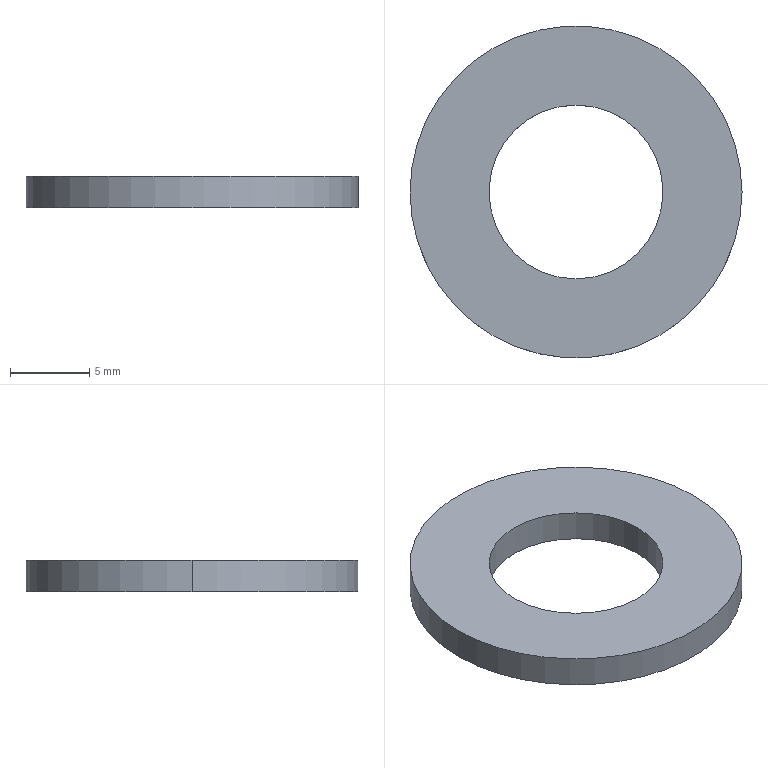Part | STEP file | Surge arrester washer | 1 solid | 6 faces | box 21 x 21 x 2 mm | volume 502.655 mm3 | cylinder 4 | plane 2 | commonest cylinder face diameters 11 x2 21 x2
STEP:
#1=CARTESIAN_POINT('',(0.,0.,0.));
#2=DIRECTION('',(0.,0.,1.));
#3=DIRECTION('',(1.,0.,0.));
#4=AXIS2_PLACEMENT_3D('',#1,#2,#3);
#5=CARTESIAN_POINT('',(-5.5,0.,2.));
#6=VERTEX_POINT('',#5);
#7=CARTESIAN_POINT('',(-5.5,0.,0.));
#8=VERTEX_POINT('',#7);
#9=CARTESIAN_POINT('',(-5.5,0.,2.));
#10=DIRECTION('',(0.,0.,-1.));
#11=VECTOR('',#10,1.);
#12=LINE('',#9,#11);
#13=CARTESIAN_POINT('',(0.,0.,2.));
#14=DIRECTION('',(0.,0.,-1.));
#15=DIRECTION('',(-1.,0.,0.));
#16=AXIS2_PLACEMENT_3D('',#13,#14,#15);
#17=CYLINDRICAL_SURFACE('',#16,5.5);
#18=CARTESIAN_POINT('',(6.283,0.));
#19=DIRECTION('',(0.,1.));
#20=VECTOR('',#19,1.);
#21=LINE('',#18,#20);
#22=(GEOMETRIC_REPRESENTATION_CONTEXT(2)PARAMETRIC_REPRESENTATION_CONTEXT()REPRESENTATION_CONTEXT('',''));
#23=DEFINITIONAL_REPRESENTATION('',(#21),#22);
#24=PCURVE('',#17,#23);
#25=CARTESIAN_POINT('',(0.,0.,2.));
#26=DIRECTION('',(0.,0.,-1.));
#27=DIRECTION('',(-1.,0.,0.));
#28=AXIS2_PLACEMENT_3D('',#25,#26,#27);
#29=CYLINDRICAL_SURFACE('',#28,5.5);
#30=CARTESIAN_POINT('',(0.,0.));
#31=DIRECTION('',(0.,1.));
#32=VECTOR('',#31,1.);
#33=LINE('',#30,#32);
#34=(GEOMETRIC_REPRESENTATION_CONTEXT(2)PARAMETRIC_REPRESENTATION_CONTEXT()REPRESENTATION_CONTEXT('',''));
#35=DEFINITIONAL_REPRESENTATION('',(#33),#34);
#36=PCURVE('',#29,#35);
#37=SURFACE_CURVE('',#12,(#24,#36),.PCURVE_S1.);
#38=EDGE_CURVE('',#6,#8,#37,.T.);
#39=ORIENTED_EDGE('',*,*,#38,.T.);
#40=CARTESIAN_POINT('',(5.5,0.,0.));
#41=VERTEX_POINT('',#40);
#42=CARTESIAN_POINT('',(0.,0.,0.));
#43=DIRECTION('',(0.,0.,1.));
#44=DIRECTION('',(1.,0.,0.));
#45=AXIS2_PLACEMENT_3D('',#42,#43,#44);
#46=CIRCLE('',#45,5.5);
#47=CARTESIAN_POINT('',(9.425,2.));
#48=DIRECTION('',(-1.,0.));
#49=VECTOR('',#48,1.);
#50=LINE('',#47,#49);
#51=(GEOMETRIC_REPRESENTATION_CONTEXT(2)PARAMETRIC_REPRESENTATION_CONTEXT()REPRESENTATION_CONTEXT('',''));
#52=DEFINITIONAL_REPRESENTATION('',(#50),#51);
#53=PCURVE('',#17,#52);
#54=CARTESIAN_POINT('',(0.,0.,0.));
#55=DIRECTION('',(0.,0.,1.));
#56=DIRECTION('',(1.,0.,0.));
#57=AXIS2_PLACEMENT_3D('',#54,#55,#56);
#58=PLANE('',#57);
#59=CARTESIAN_POINT('',(0.,0.));
#60=DIRECTION('',(1.,0.));
#61=AXIS2_PLACEMENT_2D('',#59,#60);
#62=CIRCLE('',#61,5.5);
#63=(GEOMETRIC_REPRESENTATION_CONTEXT(2)PARAMETRIC_REPRESENTATION_CONTEXT()REPRESENTATION_CONTEXT('',''));
#64=DEFINITIONAL_REPRESENTATION('',(#62),#63);
#65=PCURVE('',#58,#64);
#66=SURFACE_CURVE('',#46,(#53,#65),.PCURVE_S1.);
#67=EDGE_CURVE('',#8,#41,#66,.T.);
#68=ORIENTED_EDGE('',*,*,#67,.T.);
#69=CARTESIAN_POINT('',(5.5,0.,2.));
#70=VERTEX_POINT('',#69);
#71=CARTESIAN_POINT('',(5.5,0.,2.));
#72=DIRECTION('',(0.,0.,-1.));
#73=VECTOR('',#72,1.);
#74=LINE('',#71,#73);
#75=CARTESIAN_POINT('',(3.142,0.));
#76=DIRECTION('',(0.,1.));
#77=VECTOR('',#76,1.);
#78=LINE('',#75,#77);
#79=(GEOMETRIC_REPRESENTATION_CONTEXT(2)PARAMETRIC_REPRESENTATION_CONTEXT()REPRESENTATION_CONTEXT('',''));
#80=DEFINITIONAL_REPRESENTATION('',(#78),#79);
#81=PCURVE('',#17,#80);
#82=CARTESIAN_POINT('',(3.142,0.));
#83=DIRECTION('',(0.,1.));
#84=VECTOR('',#83,1.);
#85=LINE('',#82,#84);
#86=(GEOMETRIC_REPRESENTATION_CONTEXT(2)PARAMETRIC_REPRESENTATION_CONTEXT()REPRESENTATION_CONTEXT('',''));
#87=DEFINITIONAL_REPRESENTATION('',(#85),#86);
#88=PCURVE('',#29,#87);
#89=SURFACE_CURVE('',#74,(#81,#88),.PCURVE_S1.);
#90=EDGE_CURVE('',#70,#41,#89,.T.);
#91=ORIENTED_EDGE('',*,*,#90,.F.);
#92=CARTESIAN_POINT('',(0.,0.,2.));
#93=DIRECTION('',(0.,0.,1.));
#94=DIRECTION('',(1.,0.,0.));
#95=AXIS2_PLACEMENT_3D('',#92,#93,#94);
#96=CIRCLE('',#95,5.5);
#97=CARTESIAN_POINT('',(9.425,0.));
#98=DIRECTION('',(-1.,0.));
#99=VECTOR('',#98,1.);
#100=LINE('',#97,#99);
#101=(GEOMETRIC_REPRESENTATION_CONTEXT(2)PARAMETRIC_REPRESENTATION_CONTEXT()REPRESENTATION_CONTEXT('',''));
#102=DEFINITIONAL_REPRESENTATION('',(#100),#101);
#103=PCURVE('',#17,#102);
#104=CARTESIAN_POINT('',(0.,0.,2.));
#105=DIRECTION('',(0.,0.,1.));
#106=DIRECTION('',(1.,0.,0.));
#107=AXIS2_PLACEMENT_3D('',#104,#105,#106);
#108=PLANE('',#107);
#109=CARTESIAN_POINT('',(0.,0.));
#110=DIRECTION('',(1.,0.));
#111=AXIS2_PLACEMENT_2D('',#109,#110);
#112=CIRCLE('',#111,5.5);
#113=(GEOMETRIC_REPRESENTATION_CONTEXT(2)PARAMETRIC_REPRESENTATION_CONTEXT()REPRESENTATION_CONTEXT('',''));
#114=DEFINITIONAL_REPRESENTATION('',(#112),#113);
#115=PCURVE('',#108,#114);
#116=SURFACE_CURVE('',#96,(#103,#115),.PCURVE_S1.);
#117=EDGE_CURVE('',#6,#70,#116,.T.);
#118=ORIENTED_EDGE('',*,*,#117,.F.);
#119=EDGE_LOOP('',(#39,#68,#91,#118));
#120=FACE_BOUND('',#119,.F.);
#121=ADVANCED_FACE('',(#120),#17,.F.);
#122=CARTESIAN_POINT('',(10.5,0.,2.));
#123=VERTEX_POINT('',#122);
#124=CARTESIAN_POINT('',(-10.5,0.,2.));
#125=VERTEX_POINT('',#124);
#126=CARTESIAN_POINT('',(0.,0.,2.));
#127=DIRECTION('',(0.,0.,1.));
#128=DIRECTION('',(1.,0.,0.));
#129=AXIS2_PLACEMENT_3D('',#126,#127,#128);
#130=CIRCLE('',#129,10.5);
#131=CARTESIAN_POINT('',(0.,0.,2.));
#132=DIRECTION('',(0.,0.,-1.));
#133=DIRECTION('',(-1.,0.,0.));
#134=AXIS2_PLACEMENT_3D('',#131,#132,#133);
#135=CYLINDRICAL_SURFACE('',#134,10.5);
#136=CARTESIAN_POINT('',(3.142,0.));
#137=DIRECTION('',(-1.,0.));
#138=VECTOR('',#137,1.);
#139=LINE('',#136,#138);
#140=(GEOMETRIC_REPRESENTATION_CONTEXT(2)PARAMETRIC_REPRESENTATION_CONTEXT()REPRESENTATION_CONTEXT('',''));
#141=DEFINITIONAL_REPRESENTATION('',(#139),#140);
#142=PCURVE('',#135,#141);
#143=CARTESIAN_POINT('',(0.,0.));
#144=DIRECTION('',(1.,0.));
#145=AXIS2_PLACEMENT_2D('',#143,#144);
#146=CIRCLE('',#145,10.5);
#147=(GEOMETRIC_REPRESENTATION_CONTEXT(2)PARAMETRIC_REPRESENTATION_CONTEXT()REPRESENTATION_CONTEXT('',''));
#148=DEFINITIONAL_REPRESENTATION('',(#146),#147);
#149=PCURVE('',#108,#148);
#150=SURFACE_CURVE('',#130,(#142,#149),.PCURVE_S1.);
#151=EDGE_CURVE('',#123,#125,#150,.T.);
#152=ORIENTED_EDGE('',*,*,#151,.F.);
#153=CARTESIAN_POINT('',(10.5,0.,0.));
#154=VERTEX_POINT('',#153);
#155=CARTESIAN_POINT('',(10.5,0.,2.));
#156=DIRECTION('',(0.,0.,-1.));
#157=VECTOR('',#156,1.);
#158=LINE('',#155,#157);
#159=CARTESIAN_POINT('',(3.142,0.));
#160=DIRECTION('',(0.,1.));
#161=VECTOR('',#160,1.);
#162=LINE('',#159,#161);
#163=(GEOMETRIC_REPRESENTATION_CONTEXT(2)PARAMETRIC_REPRESENTATION_CONTEXT()REPRESENTATION_CONTEXT('',''));
#164=DEFINITIONAL_REPRESENTATION('',(#162),#163);
#165=PCURVE('',#135,#164);
#166=CARTESIAN_POINT('',(0.,0.,2.));
#167=DIRECTION('',(0.,0.,-1.));
#168=DIRECTION('',(-1.,0.,0.));
#169=AXIS2_PLACEMENT_3D('',#166,#167,#168);
#170=CYLINDRICAL_SURFACE('',#169,10.5);
#171=CARTESIAN_POINT('',(3.142,0.));
#172=DIRECTION('',(0.,1.));
#173=VECTOR('',#172,1.);
#174=LINE('',#171,#173);
#175=(GEOMETRIC_REPRESENTATION_CONTEXT(2)PARAMETRIC_REPRESENTATION_CONTEXT()REPRESENTATION_CONTEXT('',''));
#176=DEFINITIONAL_REPRESENTATION('',(#174),#175);
#177=PCURVE('',#170,#176);
#178=SURFACE_CURVE('',#158,(#165,#177),.PCURVE_S1.);
#179=EDGE_CURVE('',#123,#154,#178,.T.);
#180=ORIENTED_EDGE('',*,*,#179,.T.);
#181=CARTESIAN_POINT('',(-10.5,0.,0.));
#182=VERTEX_POINT('',#181);
#183=CARTESIAN_POINT('',(0.,0.,0.));
#184=DIRECTION('',(0.,0.,1.));
#185=DIRECTION('',(1.,0.,0.));
#186=AXIS2_PLACEMENT_3D('',#183,#184,#185);
#187=CIRCLE('',#186,10.5);
#188=CARTESIAN_POINT('',(3.142,2.));
#189=DIRECTION('',(-1.,0.));
#190=VECTOR('',#189,1.);
#191=LINE('',#188,#190);
#192=(GEOMETRIC_REPRESENTATION_CONTEXT(2)PARAMETRIC_REPRESENTATION_CONTEXT()REPRESENTATION_CONTEXT('',''));
#193=DEFINITIONAL_REPRESENTATION('',(#191),#192);
#194=PCURVE('',#135,#193);
#195=CARTESIAN_POINT('',(0.,0.));
#196=DIRECTION('',(1.,0.));
#197=AXIS2_PLACEMENT_2D('',#195,#196);
#198=CIRCLE('',#197,10.5);
#199=(GEOMETRIC_REPRESENTATION_CONTEXT(2)PARAMETRIC_REPRESENTATION_CONTEXT()REPRESENTATION_CONTEXT('',''));
#200=DEFINITIONAL_REPRESENTATION('',(#198),#199);
#201=PCURVE('',#58,#200);
#202=SURFACE_CURVE('',#187,(#194,#201),.PCURVE_S1.);
#203=EDGE_CURVE('',#154,#182,#202,.T.);
#204=ORIENTED_EDGE('',*,*,#203,.T.);
#205=CARTESIAN_POINT('',(-10.5,0.,2.));
#206=DIRECTION('',(0.,0.,-1.));
#207=VECTOR('',#206,1.);
#208=LINE('',#205,#207);
#209=CARTESIAN_POINT('',(0.,0.));
#210=DIRECTION('',(0.,1.));
#211=VECTOR('',#210,1.);
#212=LINE('',#209,#211);
#213=(GEOMETRIC_REPRESENTATION_CONTEXT(2)PARAMETRIC_REPRESENTATION_CONTEXT()REPRESENTATION_CONTEXT('',''));
#214=DEFINITIONAL_REPRESENTATION('',(#212),#213);
#215=PCURVE('',#135,#214);
#216=CARTESIAN_POINT('',(6.283,0.));
#217=DIRECTION('',(0.,1.));
#218=VECTOR('',#217,1.);
#219=LINE('',#216,#218);
#220=(GEOMETRIC_REPRESENTATION_CONTEXT(2)PARAMETRIC_REPRESENTATION_CONTEXT()REPRESENTATION_CONTEXT('',''));
#221=DEFINITIONAL_REPRESENTATION('',(#219),#220);
#222=PCURVE('',#170,#221);
#223=SURFACE_CURVE('',#208,(#215,#222),.PCURVE_S1.);
#224=EDGE_CURVE('',#125,#182,#223,.T.);
#225=ORIENTED_EDGE('',*,*,#224,.F.);
#226=EDGE_LOOP('',(#152,#180,#204,#225));
#227=FACE_BOUND('',#226,.T.);
#228=ADVANCED_FACE('',(#227),#135,.T.);
#229=CARTESIAN_POINT('',(0.,0.,2.));
#230=DIRECTION('',(0.,0.,1.));
#231=DIRECTION('',(1.,0.,0.));
#232=AXIS2_PLACEMENT_3D('',#229,#230,#231);
#233=CIRCLE('',#232,10.5);
#234=CARTESIAN_POINT('',(0.,0.));
#235=DIRECTION('',(1.,0.));
#236=AXIS2_PLACEMENT_2D('',#234,#235);
#237=CIRCLE('',#236,10.5);
#238=(GEOMETRIC_REPRESENTATION_CONTEXT(2)PARAMETRIC_REPRESENTATION_CONTEXT()REPRESENTATION_CONTEXT('',''));
#239=DEFINITIONAL_REPRESENTATION('',(#237),#238);
#240=PCURVE('',#108,#239);
#241=CARTESIAN_POINT('',(9.425,0.));
#242=DIRECTION('',(-1.,0.));
#243=VECTOR('',#242,1.);
#244=LINE('',#241,#243);
#245=(GEOMETRIC_REPRESENTATION_CONTEXT(2)PARAMETRIC_REPRESENTATION_CONTEXT()REPRESENTATION_CONTEXT('',''));
#246=DEFINITIONAL_REPRESENTATION('',(#244),#245);
#247=PCURVE('',#170,#246);
#248=SURFACE_CURVE('',#233,(#240,#247),.PCURVE_S1.);
#249=EDGE_CURVE('',#125,#123,#248,.T.);
#250=ORIENTED_EDGE('',*,*,#249,.T.);
#251=ORIENTED_EDGE('',*,*,#151,.T.);
#252=EDGE_LOOP('',(#250,#251));
#253=FACE_BOUND('',#252,.T.);
#254=ORIENTED_EDGE('',*,*,#117,.F.);
#255=CARTESIAN_POINT('',(0.,0.,2.));
#256=DIRECTION('',(0.,0.,1.));
#257=DIRECTION('',(1.,0.,0.));
#258=AXIS2_PLACEMENT_3D('',#255,#256,#257);
#259=CIRCLE('',#258,5.5);
#260=CARTESIAN_POINT('',(0.,0.));
#261=DIRECTION('',(1.,0.));
#262=AXIS2_PLACEMENT_2D('',#260,#261);
#263=CIRCLE('',#262,5.5);
#264=(GEOMETRIC_REPRESENTATION_CONTEXT(2)PARAMETRIC_REPRESENTATION_CONTEXT()REPRESENTATION_CONTEXT('',''));
#265=DEFINITIONAL_REPRESENTATION('',(#263),#264);
#266=PCURVE('',#108,#265);
#267=CARTESIAN_POINT('',(3.142,0.));
#268=DIRECTION('',(-1.,0.));
#269=VECTOR('',#268,1.);
#270=LINE('',#267,#269);
#271=(GEOMETRIC_REPRESENTATION_CONTEXT(2)PARAMETRIC_REPRESENTATION_CONTEXT()REPRESENTATION_CONTEXT('',''));
#272=DEFINITIONAL_REPRESENTATION('',(#270),#271);
#273=PCURVE('',#29,#272);
#274=SURFACE_CURVE('',#259,(#266,#273),.PCURVE_S1.);
#275=EDGE_CURVE('',#70,#6,#274,.T.);
#276=ORIENTED_EDGE('',*,*,#275,.F.);
#277=EDGE_LOOP('',(#254,#276));
#278=FACE_BOUND('',#277,.T.);
#279=ADVANCED_FACE('',(#253,#278),#108,.T.);
#280=CARTESIAN_POINT('',(0.,0.,0.));
#281=DIRECTION('',(0.,0.,1.));
#282=DIRECTION('',(1.,0.,0.));
#283=AXIS2_PLACEMENT_3D('',#280,#281,#282);
#284=CIRCLE('',#283,10.5);
#285=CARTESIAN_POINT('',(0.,0.));
#286=DIRECTION('',(1.,0.));
#287=AXIS2_PLACEMENT_2D('',#285,#286);
#288=CIRCLE('',#287,10.5);
#289=(GEOMETRIC_REPRESENTATION_CONTEXT(2)PARAMETRIC_REPRESENTATION_CONTEXT()REPRESENTATION_CONTEXT('',''));
#290=DEFINITIONAL_REPRESENTATION('',(#288),#289);
#291=PCURVE('',#58,#290);
#292=CARTESIAN_POINT('',(9.425,2.));
#293=DIRECTION('',(-1.,0.));
#294=VECTOR('',#293,1.);
#295=LINE('',#292,#294);
#296=(GEOMETRIC_REPRESENTATION_CONTEXT(2)PARAMETRIC_REPRESENTATION_CONTEXT()REPRESENTATION_CONTEXT('',''));
#297=DEFINITIONAL_REPRESENTATION('',(#295),#296);
#298=PCURVE('',#170,#297);
#299=SURFACE_CURVE('',#284,(#291,#298),.PCURVE_S1.);
#300=EDGE_CURVE('',#182,#154,#299,.T.);
#301=ORIENTED_EDGE('',*,*,#300,.F.);
#302=ORIENTED_EDGE('',*,*,#203,.F.);
#303=EDGE_LOOP('',(#301,#302));
#304=FACE_BOUND('',#303,.T.);
#305=ORIENTED_EDGE('',*,*,#67,.T.);
#306=CARTESIAN_POINT('',(0.,0.,0.));
#307=DIRECTION('',(0.,0.,1.));
#308=DIRECTION('',(1.,0.,0.));
#309=AXIS2_PLACEMENT_3D('',#306,#307,#308);
#310=CIRCLE('',#309,5.5);
#311=CARTESIAN_POINT('',(0.,0.));
#312=DIRECTION('',(1.,0.));
#313=AXIS2_PLACEMENT_2D('',#311,#312);
#314=CIRCLE('',#313,5.5);
#315=(GEOMETRIC_REPRESENTATION_CONTEXT(2)PARAMETRIC_REPRESENTATION_CONTEXT()REPRESENTATION_CONTEXT('',''));
#316=DEFINITIONAL_REPRESENTATION('',(#314),#315);
#317=PCURVE('',#58,#316);
#318=CARTESIAN_POINT('',(3.142,2.));
#319=DIRECTION('',(-1.,0.));
#320=VECTOR('',#319,1.);
#321=LINE('',#318,#320);
#322=(GEOMETRIC_REPRESENTATION_CONTEXT(2)PARAMETRIC_REPRESENTATION_CONTEXT()REPRESENTATION_CONTEXT('',''));
#323=DEFINITIONAL_REPRESENTATION('',(#321),#322);
#324=PCURVE('',#29,#323);
#325=SURFACE_CURVE('',#310,(#317,#324),.PCURVE_S1.);
#326=EDGE_CURVE('',#41,#8,#325,.T.);
#327=ORIENTED_EDGE('',*,*,#326,.T.);
#328=EDGE_LOOP('',(#305,#327));
#329=FACE_BOUND('',#328,.T.);
#330=ADVANCED_FACE('',(#304,#329),#58,.F.);
#331=ORIENTED_EDGE('',*,*,#179,.F.);
#332=ORIENTED_EDGE('',*,*,#249,.F.);
#333=ORIENTED_EDGE('',*,*,#224,.T.);
#334=ORIENTED_EDGE('',*,*,#300,.T.);
#335=EDGE_LOOP('',(#331,#332,#333,#334));
#336=FACE_BOUND('',#335,.T.);
#337=ADVANCED_FACE('',(#336),#170,.T.);
#338=ORIENTED_EDGE('',*,*,#326,.T.);
#339=ORIENTED_EDGE('',*,*,#38,.F.);
#340=ORIENTED_EDGE('',*,*,#275,.F.);
#341=ORIENTED_EDGE('',*,*,#90,.T.);
#342=EDGE_LOOP('',(#338,#339,#340,#341));
#343=FACE_BOUND('',#342,.F.);
#344=ADVANCED_FACE('',(#343),#29,.F.);
#345=CLOSED_SHELL('',(#121,#228,#279,#330,#337,#344));
#346=MANIFOLD_SOLID_BREP('',#345);
#347=(LENGTH_UNIT()NAMED_UNIT(*)SI_UNIT(.MILLI.,.METRE.));
#348=UNCERTAINTY_MEASURE_WITH_UNIT(LENGTH_MEASURE(0.0000001),#347,'','');
#349=(NAMED_UNIT(*)PLANE_ANGLE_UNIT()SI_UNIT($,.RADIAN.));
#350=(NAMED_UNIT(*)SI_UNIT($,.STERADIAN.)SOLID_ANGLE_UNIT());
#351=(GEOMETRIC_REPRESENTATION_CONTEXT(3)GLOBAL_UNCERTAINTY_ASSIGNED_CONTEXT((#348))GLOBAL_UNIT_ASSIGNED_CONTEXT((#347,#349,#350))REPRESENTATION_CONTEXT('',''));
#352=ADVANCED_BREP_SHAPE_REPRESENTATION('',(#4,#346),#351);